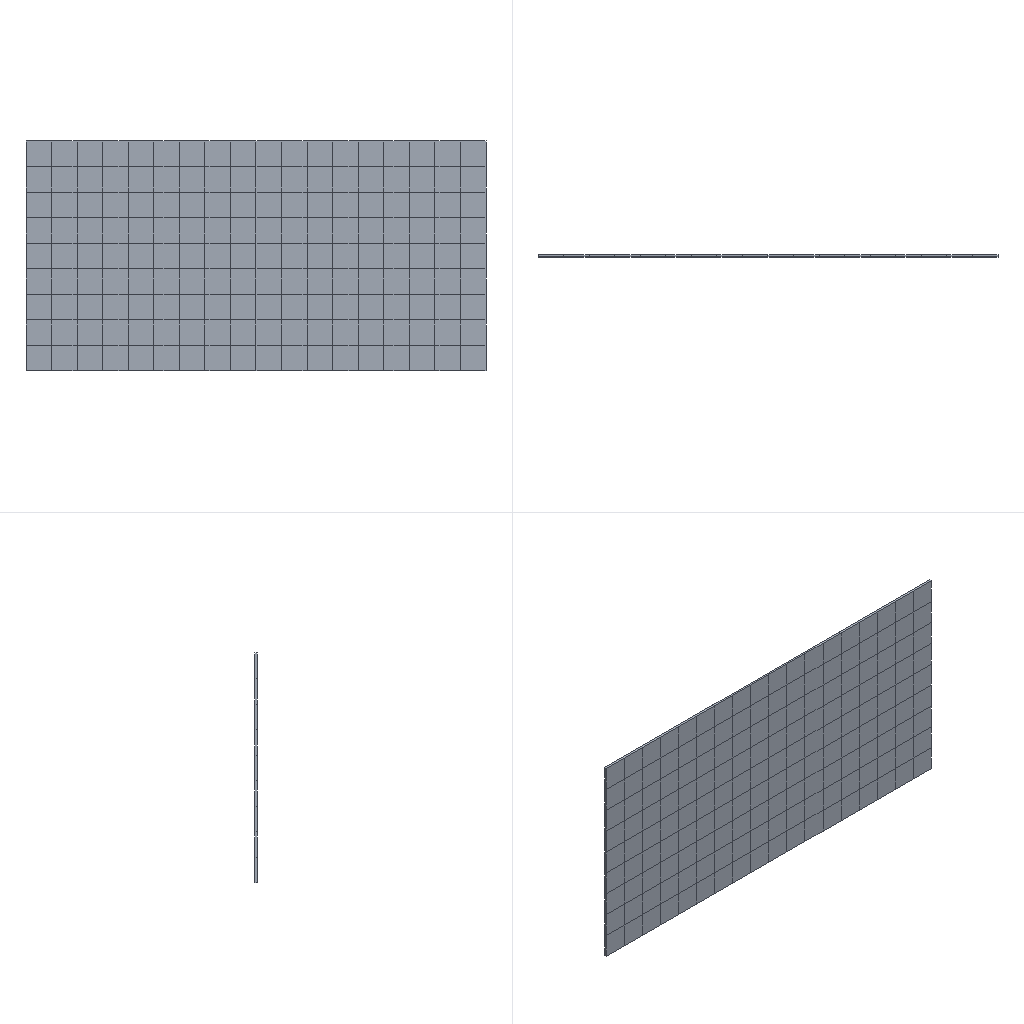Simulation study | ansys workbench
Set-up summary:
category,name,step,type,value,unit,region
solver,ansys_workbench
units,mm-N-s-tonne (MPa),,stated,"/units,MPA"
analysis,LS1,,static
load_step,LS1,LS1,static,nsubst=1; time=1
mesh,nodes,,,1272
mesh,elements,,,180
element_type,SOLID186,,,162
element_type,SURF154,,,18
material,Structural Steel,,E,200000,tonne s^-2 mm^-1
material,Structural Steel,,nu,0.3
material,Structural Steel,,density,7.85e-09,tonne mm^-3
material,Structural Steel,,conductivity,60.5,tonne mm s^-3 C^-1
material,Structural Steel,,specific_heat,4.34e+08,mm^2 s^-2 C^-1
material,Structural Steel,,cte,1.2e-05,C^-1
material,Structural Steel,,permeability,10000
material,Structural Steel,,resistivity,0.00017,ohm mm
load,Define Force Using Surface Effect Elements,LS1,surface-effect pres face 3,0.1,,SURF154 #2
bc,Fixed Supports,model,fixed,[dofs=ALL],,_FIXEDSU
named_set,_FIXEDSU,,node,48
Ansys APDL input file, long lists of numbers shortened:
/batch
/config,noeldb,1     ! force off writing results to database
*get,_wallstrt,active,,time,wall
! ANSYS input file written by Workbench version 2022 R1
! File used for geometry attach:
/title,wbnew--____ (A5)
! ****** Begin Custom Load Command Snippet ******
/COM, ACT Extensions:
/COM,     LSDYNA, 2021.1
/COM,
! ****** End   Custom Load Command Snippet ******
*DIM,_wb_ProjectScratch_dir,string,248
_wb_ProjectScratch_dir(1) = ''
*DIM,_wb_SolverFiles_dir,string,248
_wb_SolverFiles_dir(1) = ''
*DIM,_wb_userfiles_dir,string,248
_wb_userfiles_dir(1) = ''
/com,--- Data in consistent NMM units. See Solving Units in the help system for more information.
/units,MPA
/nopr
/wb,file,start              !  signify a WB generated input file
/prep7
! Turn off shape checking because checks already performed inside WB mesher.
! See help system for more information.
SHPP,OFF,,NOWARN
/nolist
etcon,set             ! allow ANSYS to choose best KEYOP's for 180x elements, resets any applicable keyopt to MAPDL defaults
/com,*********** Nodes for the whole assembly ***********
nblock,3,,1399
(1i9,3e20.9e3)
        1     8.888888889E+02     0.000000000E+00     3.888888889E+02
! (1271 more lines like these left out)
-1
/wb,elem,start            !  set before creation of elements
/com,*********** Elements for Body 1 "__-FreeParts|__-__1" ***********
et,1,186
keyo,1,2,1          ! set full integration on SOLID186
eblock,19,solid,,162
(19i9)
        1        1        1        1        0        0        0        0       20        0        1      136      353      354      355      137      300      299      298
! (323 more lines like these left out)
-1
/wb,elem,end               !  done creating elements
/com,*********** Send User Defined Coordinate System(s) ***********
csys,0
toffst,273.15,  ! Temperature offset from absolute zero
/com,*********** Set Reference Temperature ***********
tref,22.
/wb,mat,start              !  starting to send materials
/com,*********** Send Materials ***********
Temperature = 'TEMP' ! Temperature
MP,DENS,1,7.85e-09,	! tonne mm^-3
MP,ALPX,1,1.2e-05,	! C^-1
MP,C,1,434000000,	! mm^2 s^-2 C^-1
MP,KXX,1,60.5,	! tonne mm s^-3 C^-1
MP,RSVX,1,0.00017,	! ohm mm
MP,EX,1,200000,	! tonne s^-2 mm^-1
MP,NUXY,1,0.3,
MP,MURX,1,10000,
/wb,mat,end                !  done sending materials
!************************* Model Summary ********************
!__-FreeParts|__-__1,	结构钢,	matid,	1
!************************* End Model Summary ********************
! get the diagonal of the bounding box. Needed later for other things
*get,_xmin,node,,mnloc,x
*get,_ymin,node,,mnloc,y
*get,_zmin,node,,mnloc,z
*get,_xmax,node,,mxloc,x
*get,_ymax,node,,mxloc,y
*get,_zmax,node,,mxloc,z
_ASMDIAG=(_xmax-_xmin)*(_xmax-_xmin)+(_ymax-_ymin)*(_ymax-_ymin)+(_zmax-_zmin)*(_zmax-_zmin)
_ASMDIAG=SQRT(_ASMDIAG)
/wb,contact,start          !  starting to send contact
/wb,contact,end            !  done creating contacts
/golist
/wb,load,start             !  starting to send loads
/com,*********** Fixed Supports ***********
CMBLOCK,_FIXEDSU,NODE,       48
(8i10)
       290       291       292       293       294       295       296       297
       298       299       354       355       356       357       358       359
       360       361       362       363      1146      1147      1148      1149
      1150      1151      1152      1153      1154      1155      1156      1157
      1158      1159      1160      1161      1162      1163      1165      1247
      1248      1249      1250      1251      1252      1253      1254      1255
cmsel,s,_FIXEDSU
d,all,all
nsel,all
/com,*********** Define Force Using Surface Effect Elements ***********
local,12,0,0.,0.,0.,0.,0.,0.
csys,0
et,2,154
eblock,10,,,18
(15i9)
      541        2        2        2       12      299      300      353      354     1164     1167     1246     1165
! (17 more lines like these left out)
-1
esel,s,type,,2
keyop,2,2,1                ! Apply load in local coordinate system
keyop,2,7,1                ! Use original area so load is constant in large deformation
esel,all
/gst,on,on
fini
*get,_numnode,node,0,count
*get,_numelem,elem,0,count
*get, _MAXELEMNUM, elem, 0, NUM, MAX
*get, _MAXNODENUM, node, 0, NUM, MAX
*get, _MAXELEMTYPE, etyp, 0, NUM, MAX
*get, _MAXREALCONST, real, 0, NUM, MAX
/go
/wb,load,end               !  done creating loads
/com,--- Number of total nodes = %_numnode%
/com,--- Number of contact elements = 18
/com,--- Number of spring elements = 0
/com,--- Number of bearing elements = 0
/com,--- Number of solid elements = 162
/com,--- Number of condensed parts = 0
/com,--- Number of total elements = %_numelem%
*get,_wallbsol,active,,time,wall
/com,****************************************************************************
/com,*************************    SOLUTION       ********************************
/com,****************************************************************************
/solu
antype,0                   ! static analysis
_thickRatio=  0     ! Ratio of thick parts in the model
eqsl,sparse,,,,,1
cntr,print,1               ! print out contact info and also make no initial contact an error
dmpoption,emat,no             ! Don't combine emat file for DANSYS
dmpoption,esav,no             ! Don't combine esav file for DANSYS
nldiag,cont,iter           ! print out contact info each equilibrium iteration
rescontrol,,none                 ! Do not keep any restart files
/com,****************************************************
/com,******************* SOLVE FOR LS 1 OF 1 ****************
esel,s,type,,2
nsle
sfe,all,1,pres,1,0.
sfe,all,2,pres,1,0.
sfe,all,3,pres,1,0.1
nsel,all
esel,all
/nopr
/gopr
nsub,1,1,1
time,1.
outres,erase
outres,all,none
outres,nsol,all,
outres,rsol,all
outres,eangl,all
outres,etmp,all
outres,veng,all
outres,strs,all,
outres,epel,all,
outres,eppl,all,
outres,cont,all,
! *********** WB SOLVE COMMAND ***********
! check interactive state
*get,ANSINTER_,active,,int
*if,ANSINTER_,ne,0,then
/eof
*endif
solve
/com *************** Write FE CONNECTORS *********
CEWRITE,file,ce,,INTE
/com,****************************************************
/com,*************** FINISHED SOLVE FOR LS 1 *************
*get,_wallasol,active,,time,wall
/nopr
*get,_numnode,node,0,count
*get,_numelem,elem,0,count
*get, _MAXELEMNUM, elem, 0, NUM, MAX
*get, _MAXNODENUM, node, 0, NUM, MAX,,,INTERNAL
*get, _MAXELEMTYPE, etyp, 0, NUM, MAX
*get, _MAXREALCONST, real, 0, NUM, MAX
/gopr
/post1
xmlo,ENCODING,ISO-8859-1
xmlo,parm
/xml,parm,xml
fini
/gopr
*get,_walldone,active,,time,wall
_preptime=(_wallbsol-_wallstrt)*3600
_solvtime=(_wallasol-_wallbsol)*3600
_posttime=(_walldone-_wallasol)*3600
_totaltim=(_walldone-_wallstrt)*3600
*get,_dlbratio,active,0,solu,dlbr
*get,_combtime,active,0,solu,comb
*get,_ssmode,active,0,solu,ssmm
*get,_ndofs,active,0,solu,ndof
*get,_sol_end_time,active,0,set,time
*if,_sol_end_time,eq,1.,then
/fclean				!clean distributed files
*endif
/com,--- Total number of nodes = %_numnode%
/com,--- Total number of elements = %_numelem%
/com,--- Element load balance ratio = %_dlbratio%
/com,--- Time to combine distributed files = %_combtime%
/com,--- Sparse memory mode = %_ssmode%
/com,--- Number of DOF = %_ndofs%
/wb,file,end               ! done with WB generated input
Results summary:
result,analyses[0].index,,,1
result,analyses[0].system,,,SYS
result,analyses[0].deck,,,deck.dat
result,analyses[0].solve_status,,,completed
result,analyses[0].analysis_type,,,static
result,analyses[0].physics,,,mechanical
result,analyses[0].unit_system,,,"NMM: mm, ton, N, s, mV, mA, degC"
result,analyses[0].n_sets,,,1
result,analyses[0].load_steps[0].set,set=1,,1
result,analyses[0].load_steps[0].time_or_freq,set=1,,1
result,analyses[0].load_steps[0].max_displacement_magnitude,set=1,,0.01596
result,analyses[0].load_steps[0].max_von_mises_nodal,set=1,,1.852
result,analyses[0].load_steps[0].reaction_force_sum_xyz[1],set=1,,2.38799e-09
result,analyses[0].load_steps[0].reaction_force_sum_xyz[2],set=1,,1.21788e-08
result,analyses[0].load_steps[0].reaction_force_sum_xyz[3],set=1,,-2000